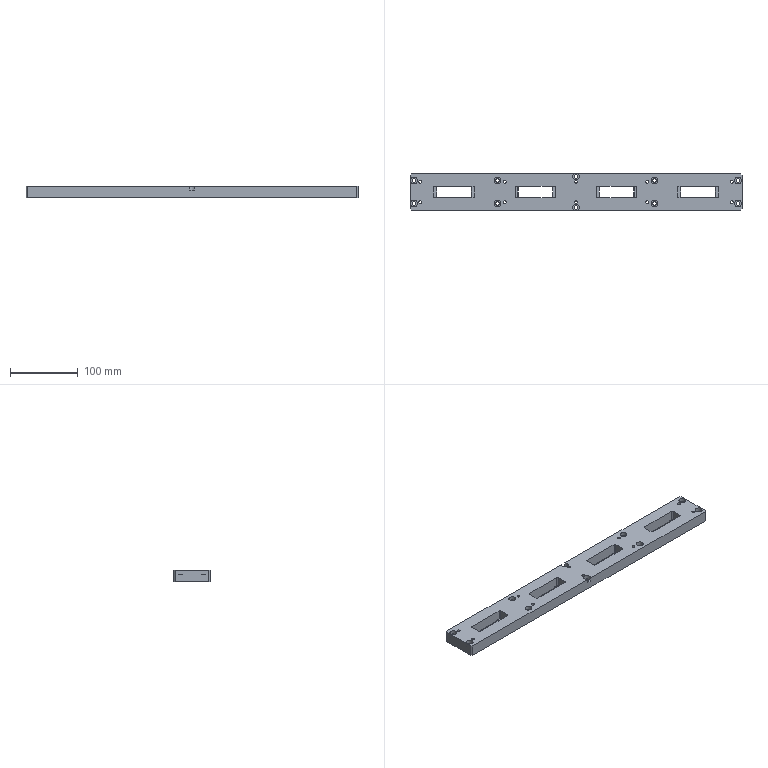NC program | NX | posted with a generic post | part box 490 x 54 x 17 mm
Whole program:
N10 G17 G21 G94 G90
(FLOOR_WALL_COPY , TOOL : D80)
N12 T19 M6
N14 G54
N16 G17 G0 G90 X-43. Y-27. S6500 M3
N18 G43 Z30. H19
N20 Z5.
N22 G94 G1 Z2. F1500.
N24 X-40.
N26 X530.
N28 X533.
N30 Z5.
N32 G0 Z30.
N34 X-43.
N36 Z4.
N38 G1 Z1.
N40 X-40.
N42 X530.
N44 X533.
N46 Z4.
N48 G0 Z30.
N50 X-43.
N52 Z3.
N54 G1 Z0.
N56 X-40.
N58 X530.
N60 X533.
N62 Z3.
N64 G0 Z30.
N66 M5
(HOLE_MILLING_1 , TOOL : D3)
N68 T03 M6
N70 G54
N72 G17 G0 G90 X5. Y-27. S9500 M3
N74 G43 Z30. H3
N76 Z0.5
N78 G94 G3 X4.55 Y-26.55 R0.45 F1000.
N80 X4.1 Y-27. R0.45
N82 X4.1 Y-27. Z0.2 I0.9 J0.
N84 X4.1 Y-27. Z-0.1 I0.9 J0.
N86 X4.1 Y-27. Z-0.4 I0.9 J0.
N88 X4.1 Y-27. Z-0.7 I0.9 J0.
N90 X4.1 Y-27. Z-1. I0.9 J0.
N92 X4.1 Y-27. Z-1.3 I0.9 J0.
N94 X4.1 Y-27. Z-1.6 I0.9 J0.
N96 X4.1 Y-27. Z-1.9 I0.9 J0.
N98 X4.1 Y-27. Z-2.2 I0.9 J0.
N100 X4.1 Y-27. Z-2.5 I0.9 J0.
N102 X4.1 Y-27. Z-2.8 I0.9 J0.
N104 X4.1 Y-27. Z-3.1 I0.9 J0.
N106 X4.1 Y-27. Z-3.4 I0.9 J0.
N108 X4.1 Y-27. Z-3.7 I0.9 J0.
N110 X4.1 Y-27. Z-4. I0.9 J0.
N112 X4.1 Y-27. Z-4.3 I0.9 J0.
N114 X4.1 Y-27. Z-4.6 I0.9 J0.
N116 X4.1 Y-27. Z-4.9 I0.9 J0.
N118 X4.1 Y-27. Z-5.2 I0.9 J0.
N120 X4.1 Y-27. Z-5.5 I0.9 J0.
N122 X4.1 Y-27. Z-5.8 I0.9 J0.
N124 X4.1 Y-27. Z-6.1 I0.9 J0.
N126 X4.1 Y-27. Z-6.4 I0.9 J0.
N128 X4.1 Y-27. Z-6.7 I0.9 J0.
N130 X4.1 Y-27. Z-7. I0.9 J0.
N132 X4.1 Y-27. Z-7.3 I0.9 J0.
N134 X4.1 Y-27. Z-7.6 I0.9 J0.
N136 X4.1 Y-27. Z-7.9 I0.9 J0.
N138 X4.1 Y-27. Z-8.2 I0.9 J0.
N140 X4.1 Y-27. Z-8.5 I0.9 J0.
N142 X4.1 Y-27. Z-8.8 I0.9 J0.
N144 X4.1 Y-27. Z-9.1 I0.9 J0.
N146 X4.1 Y-27. Z-9.4 I0.9 J0.
N148 X4.1 Y-27. Z-9.7 I0.9 J0.
N150 X4.1 Y-27. Z-10. I0.9 J0.
N152 X5. Y-27.9 R0.9
N154 X4.1 Y-27. R-0.9
N156 X4.55 Y-27.45 R0.45
N158 X5. Y-27. R0.45
N160 G0 Z30.
N162 X485.
N164 Z0.5
N166 G3 X484.55 Y-26.55 R0.45
N168 X484.1 Y-27. R0.45
N170 X484.1 Y-27. Z0.2 I0.9 J0.
N172 X484.1 Y-27. Z-0.1 I0.9 J0.
N174 X484.1 Y-27. Z-0.4 I0.9 J0.
N176 X484.1 Y-27. Z-0.7 I0.9 J0.
N178 X484.1 Y-27. Z-1. I0.9 J0.
N180 X484.1 Y-27. Z-1.3 I0.9 J0.
N182 X484.1 Y-27. Z-1.6 I0.9 J0.
N184 X484.1 Y-27. Z-1.9 I0.9 J0.
N186 X484.1 Y-27. Z-2.2 I0.9 J0.
N188 X484.1 Y-27. Z-2.5 I0.9 J0.
N190 X484.1 Y-27. Z-2.8 I0.9 J0.
N192 X484.1 Y-27. Z-3.1 I0.9 J0.
N194 X484.1 Y-27. Z-3.4 I0.9 J0.
N196 X484.1 Y-27. Z-3.7 I0.9 J0.
N198 X484.1 Y-27. Z-4. I0.9 J0.
N200 X484.1 Y-27. Z-4.3 I0.9 J0.
N202 X484.1 Y-27. Z-4.6 I0.9 J0.
N204 X484.1 Y-27. Z-4.9 I0.9 J0.
N206 X484.1 Y-27. Z-5.2 I0.9 J0.
N208 X484.1 Y-27. Z-5.5 I0.9 J0.
N210 X484.1 Y-27. Z-5.8 I0.9 J0.
N212 X484.1 Y-27. Z-6.1 I0.9 J0.
N214 X484.1 Y-27. Z-6.4 I0.9 J0.
N216 X484.1 Y-27. Z-6.7 I0.9 J0.
N218 X484.1 Y-27. Z-7. I0.9 J0.
N220 X484.1 Y-27. Z-7.3 I0.9 J0.
N222 X484.1 Y-27. Z-7.6 I0.9 J0.
N224 X484.1 Y-27. Z-7.9 I0.9 J0.
N226 X484.1 Y-27. Z-8.2 I0.9 J0.
N228 X484.1 Y-27. Z-8.5 I0.9 J0.
N230 X484.1 Y-27. Z-8.8 I0.9 J0.
N232 X484.1 Y-27. Z-9.1 I0.9 J0.
N234 X484.1 Y-27. Z-9.4 I0.9 J0.
N236 X484.1 Y-27. Z-9.7 I0.9 J0.
N238 X484.1 Y-27. Z-10. I0.9 J0.
N240 X485. Y-27.9 R0.9
N242 X484.1 Y-27. R-0.9
N244 X484.55 Y-27.45 R0.45
N246 X485. Y-27. R0.45
N248 G0 Z30.
N250 M5
(PLANAR_MILL_COPY_COPY , TOOL : D6A45)
N252 T01 M6
N254 G54
N256 G17 G0 G90 X475.866 Y-11.3 S9500 M3
N258 G43 Z30. H1
N260 Z0.5
N262 G94 G1 Z-1. F1250.
N264 G3 X475. Y-10.8 R1.
N266 X473.8 Y-12. R1.2
N268 X475. Y-10.8 R-1.2
N270 X474.134 Y-11.3 R1.
N272 G1 Z0.5
N274 G0 Z30.
N276 X485.35 Y-10.866
N278 Z0.5
N280 G1 Z-1.
N282 G3 X485.85 Y-10. R1.
N284 X484. Y-8.15 R1.85
N286 X485.85 Y-10. R-1.85
N288 X485.35 Y-9.134 R1.
N290 G1 Z0.5
N292 G0 Z30.
N294 X486.1 Y-27.866
N296 Z0.5
N298 G1 Z-1.
N300 G3 X486.6 Y-27. R1.
N302 X485. Y-25.4 R1.6
N304 X486.6 Y-27. R-1.6
N306 X486.1 Y-26.134 R1.
N308 G1 Z0.5
N310 G0 Z30.
N312 X485.35 Y-44.866
N314 Z0.5
N316 G1 Z-1.
N318 G3 X485.85 Y-44. R1.
N320 X484. Y-42.15 R1.85
N322 X485.85 Y-44. R-1.85
N324 X485.35 Y-43.134 R1.
N326 G1 Z0.5
N328 G0 Z30.
N330 X474.134 Y-42.7
N332 Z0.5
N334 G1 Z-1.
N336 G3 X475. Y-43.2 R1.
N338 X476.2 Y-42. R1.2
N340 X475. Y-43.2 R-1.2
N342 X475.866 Y-42.7 R1.
N344 G1 Z0.5
N346 G0 Z30.
N348 X360.134 Y-45.35
N350 Z0.5
N352 G1 Z-1.
N354 G3 X361. Y-45.85 R1.
N356 X362.85 Y-44. R1.85
N358 X361. Y-45.85 R-1.85
N360 X361.866 Y-45.35 R1.
N362 G1 Z0.5
N364 G0 Z30.
N366 X349.134 Y-42.7
N368 Z0.5
N370 G1 Z-1.
N372 G3 X350. Y-43.2 R1.
N374 X351.2 Y-42. R1.2
N376 X350. Y-43.2 R-1.2
N378 X350.866 Y-42.7 R1.
N380 G1 Z0.5
N382 G0 Z30.
N384 X361.866 Y-8.65
N386 Z0.5
N388 G1 Z-1.
N390 G3 X361. Y-8.15 R1.
N392 X359.15 Y-10. R1.85
N394 X361. Y-8.15 R-1.85
N396 X360.134 Y-8.65 R1.
N398 G1 Z0.5
N400 G0 Z30.
N402 X350.866 Y-11.3
N404 Z0.5
N406 G1 Z-1.
N408 G3 X350. Y-10.8 R1.
N410 X348.8 Y-12. R1.2
N412 X350. Y-10.8 R-1.2
N414 X349.134 Y-11.3 R1.
N416 G1 Z0.5
N418 G0 Z30.
N420 X245.866 Y-2.65
N422 Z0.5
N424 G1 Z-1.
N426 G3 X245. Y-2.15 R1.
N428 X243.15 Y-4. R1.85
N430 X245. Y-2.15 R-1.85
N432 X244.134 Y-2.65 R1.
N434 G1 Z0.5
N436 G0 Z30.
N438 X245.866 Y-11.3
N440 Z0.5
N442 G1 Z-1.
N444 G3 X245. Y-10.8 R1.
N446 X243.8 Y-12. R1.2
N448 X245. Y-10.8 R-1.2
N450 X244.134 Y-11.3 R1.
N452 G1 Z0.5
N454 G0 Z30.
N456 Y1.4
N458 Z0.5
N460 G1 Z-1.
N462 G3 X245. Y0.9 R1.
N464 G1 X488.
N466 G2 X488.636 Y0.636 R0.9
N468 G1 X490.636 Y-1.364
N470 G2 X490.9 Y-2. R0.9
N472 G1 Y-52.
N474 G2 X490.636 Y-52.636 R0.9
N476 G1 X488.636 Y-54.636
N478 G2 X488. Y-54.9 R0.9
N480 G1 X2.
N482 G2 X1.364 Y-54.636 R0.9
N484 G1 X-0.636 Y-52.636
N486 G2 X-0.9 Y-52. R0.9
N488 G1 Y-2.
N490 G2 X-0.636 Y-1.364 R0.9
N492 G1 X1.364 Y0.636
N494 G2 X2. Y0.9 R0.9
N496 G1 X245.
N498 G3 X245.866 Y1.4 R1.
N500 G1 Z0.5
N502 G0 Z30.
N504 X244.134 Y-42.7
N506 Z0.5
N508 G1 Z-1.
N510 G3 X245. Y-43.2 R1.
N512 X246.2 Y-42. R1.2
N514 X245. Y-43.2 R-1.2
N516 X245.866 Y-42.7 R1.
N518 G1 Z0.5
N520 G0 Z30.
N522 X244.134 Y-51.35
N524 Z0.5
N526 G1 Z-1.
N528 G3 X245. Y-51.85 R1.
N530 X246.85 Y-50. R1.85
N532 X245. Y-51.85 R-1.85
N534 X245.866 Y-51.35 R1.
N536 G1 Z0.5
N538 G0 Z30.
N540 X139.134 Y-42.7
N542 Z0.5
N544 G1 Z-1.
N546 G3 X140. Y-43.2 R1.
N548 X141.2 Y-42. R1.2
N550 X140. Y-43.2 R-1.2
N552 X140.866 Y-42.7 R1.
N554 G1 Z0.5
N556 G0 Z30.
N558 X128.134 Y-45.35
N560 Z0.5
N562 G1 Z-1.
N564 G3 X129. Y-45.85 R1.
N566 X130.85 Y-44. R1.85
N568 X129. Y-45.85 R-1.85
N570 X129.866 Y-45.35 R1.
N572 G1 Z0.5
N574 G0 Z30.
N576 X140.866 Y-11.3
N578 Z0.5
N580 G1 Z-1.
N582 G3 X140. Y-10.8 R1.
N584 X138.8 Y-12. R1.2
N586 X140. Y-10.8 R-1.2
N588 X139.134 Y-11.3 R1.
N590 G1 Z0.5
N592 G0 Z30.
N594 X129.866 Y-8.65
N596 Z0.5
N598 G1 Z-1.
N600 G3 X129. Y-8.15 R1.
N602 X127.15 Y-10. R1.85
N604 X129. Y-8.15 R-1.85
N606 X128.134 Y-8.65 R1.
N608 G1 Z0.5
N610 G0 Z30.
N612 X15.866 Y-11.3
N614 Z0.5
N616 G1 Z-1.
N618 G3 X15. Y-10.8 R1.
N620 X13.8 Y-12. R1.2
N622 X15. Y-10.8 R-1.2
N624 X14.134 Y-11.3 R1.
N626 G1 Z0.5
N628 G0 Z30.
N630 X4.65 Y-9.134
N632 Z0.5
N634 G1 Z-1.
N636 G3 X4.15 Y-10. R1.
N638 X6. Y-11.85 R1.85
N640 X4.15 Y-10. R-1.85
N642 X4.65 Y-10.866 R1.
N644 G1 Z0.5
N646 G0 Z30.
N648 X3.9 Y-26.134
N650 Z0.5
N652 G1 Z-1.
N654 G3 X3.4 Y-27. R1.
N656 X5. Y-28.6 R1.6
N658 X3.4 Y-27. R-1.6
N660 X3.9 Y-27.866 R1.
N662 G1 Z0.5
N664 G0 Z30.
N666 X4.65 Y-43.134
N668 Z0.5
N670 G1 Z-1.
N672 G3 X4.15 Y-44. R1.
N674 X6. Y-45.85 R1.85
N676 X4.15 Y-44. R-1.85
N678 X4.65 Y-44.866 R1.
N680 G1 Z0.5
N682 G0 Z30.
N684 X14.134 Y-42.7
N686 Z0.5
N688 G1 Z-1.
N690 G3 X15. Y-43.2 R1.
N692 X16.2 Y-42. R1.2
N694 X15. Y-43.2 R-1.2
N696 X15.866 Y-42.7 R1.
N698 G1 Z0.5
N700 G0 Z30.
(PLANAR_MILL_COPY_COPY_COPY , TOOL : D6A45)
N702 X65.866 Y-19.4
N704 Z0.
N706 G1 Z-1.5
N708 G3 X65. Y-18.9 R1.
N710 G1 X41.5
N712 G3 X40. Y-20.4 R1.5
N714 G1 Y-33.6
N716 G3 X41.5 Y-35.1 R1.5
N718 G1 X88.5
N720 G3 X90. Y-33.6 R1.5
N722 G1 Y-20.4
N724 G3 X88.5 Y-18.9 R1.5
N726 G1 X65.
N728 G3 X64.134 Y-19.4 R1.
N730 G1 Z0.
N732 G0 Z30.
N734 X185.866
N736 Z0.
N738 G1 Z-1.5
N740 G3 X185. Y-18.9 R1.
N742 G1 X161.5
N744 G3 X160. Y-20.4 R1.5
N746 G1 Y-33.6
N748 G3 X161.5 Y-35.1 R1.5
N750 G1 X208.5
N752 G3 X210. Y-33.6 R1.5
N754 G1 Y-20.4
N756 G3 X208.5 Y-18.9 R1.5
N758 G1 X185.
N760 G3 X184.134 Y-19.4 R1.
N762 G1 Z0.
N764 G0 Z30.
N766 X305.866
N768 Z0.
N770 G1 Z-1.5
N772 G3 X305. Y-18.9 R1.
N774 G1 X281.5
N776 G3 X280. Y-20.4 R1.5
N778 G1 Y-33.6
N780 G3 X281.5 Y-35.1 R1.5
N782 G1 X328.5
N784 G3 X330. Y-33.6 R1.5
N786 G1 Y-20.4
N788 G3 X328.5 Y-18.9 R1.5
N790 G1 X305.
N792 G3 X304.134 Y-19.4 R1.
N794 G1 Z0.
N796 G0 Z30.
N798 X425.866
N800 Z0.
N802 G1 Z-1.5
N804 G3 X425. Y-18.9 R1.
N806 G1 X401.5
N808 G3 X400. Y-20.4 R1.5
N810 G1 Y-33.6
N812 G3 X401.5 Y-35.1 R1.5
N814 G1 X448.5
N816 G3 X450. Y-33.6 R1.5
N818 G1 Y-20.4
N820 G3 X448.5 Y-18.9 R1.5
N822 G1 X425.
N824 G3 X424.134 Y-19.4 R1.
N826 G1 Z0.
N828 G0 Z30.
N830 M5
(刀补 , TOOL : D3)
N832 T03 M6
N834 G54
N836 G17 G0 G90 X5. Y-27. S9500 M3
N838 G43 Z30. H3
N840 Z0.5
N842 G41 G94 G1 X4.996 Y-26.9 F1000. D3
N844 G3 X4.05 Y-27. R0.478
N846 X4.05 Y-27. Z-1.5 I0.95 J0.
N848 X4.05 Y-27. Z-3.5 I0.95 J0.
N850 X4.05 Y-27. Z-5.5 I0.95 J0.
N852 X4.05 Y-27. Z-7.5 I0.95 J0.
N854 X4.05 Y-27. Z-9.5 I0.95 J0.
N856 X5. Y-27.95 Z-10. R0.95
N858 X5.95 Y-27. R0.95
N860 X5. Y-27.95 R-0.95
N862 X5.1 Y-27.004 R0.478
N864 G40
N866 G1 X5. Y-27.
N868 G0 Z30.
N870 X485.
N872 Z0.5
N874 G41 G1 X484.996 Y-26.9
N876 G3 X484.05 Y-27. R0.478
N878 X484.05 Y-27. Z-1.5 I0.95 J0.
N880 X484.05 Y-27. Z-3.5 I0.95 J0.
N882 X484.05 Y-27. Z-5.5 I0.95 J0.
N884 X484.05 Y-27. Z-7.5 I0.95 J0.
N886 X484.05 Y-27. Z-9.5 I0.95 J0.
N888 X485. Y-27.95 Z-10. R0.95
N890 X485.95 Y-27. R0.95
N892 X485. Y-27.95 R-0.95
N894 X485.1 Y-27.004 R0.478
N896 G40
N898 G1 X485. Y-27.
N900 G0 Z30.
N902 M5
N904 M2